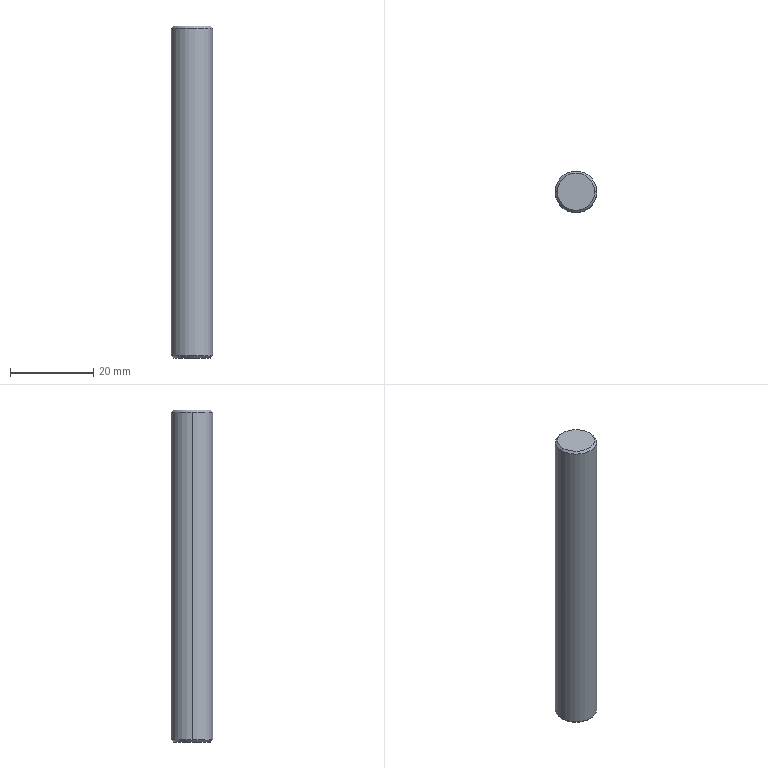Part | SolidWorks | features Chamfer 1, Extrusion 1 | 1 solid | 8 faces | box 10 x 10 x 80 mm | volume 6276 mm3 | cone 4 | cylinder 2 | plane 2 | commonest cylinder face diameters 10 x2
STEP:
#1=CARTESIAN_POINT('',(4.5,0.,80.));
#2=VERTEX_POINT('',#1);
#3=CARTESIAN_POINT('',(-4.5,0.,80.));
#4=VERTEX_POINT('',#3);
#5=CARTESIAN_POINT('',(0.,0.,80.));
#6=DIRECTION('',(0.,0.,1.));
#7=DIRECTION('',(1.,0.,0.));
#8=AXIS2_PLACEMENT_3D('',#5,#6,#7);
#9=CIRCLE('',#8,4.5);
#10=EDGE_CURVE('',#2,#4,#9,.T.);
#11=ORIENTED_EDGE('',*,*,#10,.F.);
#12=CARTESIAN_POINT('',(5.,0.,79.5));
#13=VERTEX_POINT('',#12);
#14=CARTESIAN_POINT('',(4.5,0.,80.));
#15=DIRECTION('',(0.7071,0.,-0.7071));
#16=VECTOR('',#15,1000.);
#17=LINE('',#14,#16);
#18=EDGE_CURVE('',#2,#13,#17,.T.);
#19=ORIENTED_EDGE('',*,*,#18,.T.);
#20=CARTESIAN_POINT('',(-5.,0.,79.5));
#21=VERTEX_POINT('',#20);
#22=CARTESIAN_POINT('',(0.,0.,79.5));
#23=DIRECTION('',(0.,0.,-1.));
#24=DIRECTION('',(1.,0.,0.));
#25=AXIS2_PLACEMENT_3D('',#22,#23,#24);
#26=CIRCLE('',#25,5.);
#27=EDGE_CURVE('',#21,#13,#26,.T.);
#28=ORIENTED_EDGE('',*,*,#27,.F.);
#29=CARTESIAN_POINT('',(-4.5,0.,80.));
#30=DIRECTION('',(-0.7071,0.,-0.7071));
#31=VECTOR('',#30,1000.);
#32=LINE('',#29,#31);
#33=EDGE_CURVE('',#4,#21,#32,.T.);
#34=ORIENTED_EDGE('',*,*,#33,.F.);
#35=EDGE_LOOP('',(#11,#19,#28,#34));
#36=FACE_OUTER_BOUND('',#35,.T.);
#37=CARTESIAN_POINT('',(0.,0.,80.));
#38=DIRECTION('',(0.,0.,-1.));
#39=DIRECTION('',(-1.,0.,0.));
#40=AXIS2_PLACEMENT_3D('',#37,#38,#39);
#41=CONICAL_SURFACE('',#40,4.5,0.7854);
#42=ADVANCED_FACE('',(#36),#41,.T.);
#43=CARTESIAN_POINT('',(-4.5,0.,0.));
#44=VERTEX_POINT('',#43);
#45=CARTESIAN_POINT('',(4.5,0.,0.));
#46=VERTEX_POINT('',#45);
#47=CARTESIAN_POINT('',(0.,0.,0.));
#48=DIRECTION('',(0.,0.,-1.));
#49=DIRECTION('',(1.,0.,0.));
#50=AXIS2_PLACEMENT_3D('',#47,#48,#49);
#51=CIRCLE('',#50,4.5);
#52=EDGE_CURVE('',#44,#46,#51,.T.);
#53=ORIENTED_EDGE('',*,*,#52,.F.);
#54=CARTESIAN_POINT('',(-5.,0.,0.5));
#55=VERTEX_POINT('',#54);
#56=CARTESIAN_POINT('',(-5.,0.,0.5));
#57=DIRECTION('',(-0.7071,0.,0.7071));
#58=VECTOR('',#57,1000.);
#59=LINE('',#56,#58);
#60=EDGE_CURVE('',#44,#55,#59,.T.);
#61=ORIENTED_EDGE('',*,*,#60,.T.);
#62=CARTESIAN_POINT('',(5.,0.,0.5));
#63=VERTEX_POINT('',#62);
#64=CARTESIAN_POINT('',(0.,0.,0.5));
#65=DIRECTION('',(0.,0.,1.));
#66=DIRECTION('',(1.,0.,0.));
#67=AXIS2_PLACEMENT_3D('',#64,#65,#66);
#68=CIRCLE('',#67,5.);
#69=EDGE_CURVE('',#63,#55,#68,.T.);
#70=ORIENTED_EDGE('',*,*,#69,.F.);
#71=CARTESIAN_POINT('',(5.,0.,0.5));
#72=DIRECTION('',(0.7071,0.,0.7071));
#73=VECTOR('',#72,1000.);
#74=LINE('',#71,#73);
#75=EDGE_CURVE('',#46,#63,#74,.T.);
#76=ORIENTED_EDGE('',*,*,#75,.F.);
#77=EDGE_LOOP('',(#53,#61,#70,#76));
#78=FACE_OUTER_BOUND('',#77,.T.);
#79=CARTESIAN_POINT('',(0.,0.,0.5));
#80=DIRECTION('',(0.,0.,1.));
#81=DIRECTION('',(1.,0.,0.));
#82=AXIS2_PLACEMENT_3D('',#79,#80,#81);
#83=CONICAL_SURFACE('',#82,5.,0.7854);
#84=ADVANCED_FACE('',(#78),#83,.T.);
#85=ORIENTED_EDGE('',*,*,#27,.T.);
#86=CARTESIAN_POINT('',(5.,0.,80.));
#87=DIRECTION('',(0.,0.,-1.));
#88=VECTOR('',#87,1000.);
#89=LINE('',#86,#88);
#90=EDGE_CURVE('',#13,#63,#89,.T.);
#91=ORIENTED_EDGE('',*,*,#90,.T.);
#92=ORIENTED_EDGE('',*,*,#69,.T.);
#93=CARTESIAN_POINT('',(-5.,0.,80.));
#94=DIRECTION('',(0.,0.,-1.));
#95=VECTOR('',#94,1000.);
#96=LINE('',#93,#95);
#97=EDGE_CURVE('',#21,#55,#96,.T.);
#98=ORIENTED_EDGE('',*,*,#97,.F.);
#99=EDGE_LOOP('',(#85,#91,#92,#98));
#100=FACE_OUTER_BOUND('',#99,.T.);
#101=CARTESIAN_POINT('',(0.,0.,80.));
#102=DIRECTION('',(0.,0.,-1.));
#103=DIRECTION('',(-1.,0.,0.));
#104=AXIS2_PLACEMENT_3D('',#101,#102,#103);
#105=CYLINDRICAL_SURFACE('',#104,5.);
#106=ADVANCED_FACE('',(#100),#105,.T.);
#107=ORIENTED_EDGE('',*,*,#90,.F.);
#108=CARTESIAN_POINT('',(0.,0.,79.5));
#109=DIRECTION('',(0.,0.,-1.));
#110=DIRECTION('',(1.,0.,0.));
#111=AXIS2_PLACEMENT_3D('',#108,#109,#110);
#112=CIRCLE('',#111,5.);
#113=EDGE_CURVE('',#13,#21,#112,.T.);
#114=ORIENTED_EDGE('',*,*,#113,.T.);
#115=ORIENTED_EDGE('',*,*,#97,.T.);
#116=CARTESIAN_POINT('',(0.,0.,0.5));
#117=DIRECTION('',(0.,0.,1.));
#118=DIRECTION('',(1.,0.,0.));
#119=AXIS2_PLACEMENT_3D('',#116,#117,#118);
#120=CIRCLE('',#119,5.);
#121=EDGE_CURVE('',#55,#63,#120,.T.);
#122=ORIENTED_EDGE('',*,*,#121,.T.);
#123=EDGE_LOOP('',(#107,#114,#115,#122));
#124=FACE_OUTER_BOUND('',#123,.T.);
#125=CARTESIAN_POINT('',(0.,0.,80.));
#126=DIRECTION('',(0.,0.,-1.));
#127=DIRECTION('',(-1.,0.,0.));
#128=AXIS2_PLACEMENT_3D('',#125,#126,#127);
#129=CYLINDRICAL_SURFACE('',#128,5.);
#130=ADVANCED_FACE('',(#124),#129,.T.);
#131=CARTESIAN_POINT('',(0.,0.,80.));
#132=DIRECTION('',(0.,0.,1.));
#133=DIRECTION('',(1.,0.,0.));
#134=AXIS2_PLACEMENT_3D('',#131,#132,#133);
#135=CIRCLE('',#134,4.5);
#136=EDGE_CURVE('',#4,#2,#135,.T.);
#137=ORIENTED_EDGE('',*,*,#136,.T.);
#138=ORIENTED_EDGE('',*,*,#10,.T.);
#139=EDGE_LOOP('',(#137,#138));
#140=FACE_OUTER_BOUND('',#139,.T.);
#141=CARTESIAN_POINT('',(0.,0.,80.));
#142=DIRECTION('',(0.,0.,1.));
#143=DIRECTION('',(1.,0.,0.));
#144=AXIS2_PLACEMENT_3D('',#141,#142,#143);
#145=PLANE('',#144);
#146=ADVANCED_FACE('',(#140),#145,.T.);
#147=CARTESIAN_POINT('',(0.,0.,0.));
#148=DIRECTION('',(0.,0.,-1.));
#149=DIRECTION('',(1.,0.,0.));
#150=AXIS2_PLACEMENT_3D('',#147,#148,#149);
#151=CIRCLE('',#150,4.5);
#152=EDGE_CURVE('',#46,#44,#151,.T.);
#153=ORIENTED_EDGE('',*,*,#152,.T.);
#154=ORIENTED_EDGE('',*,*,#52,.T.);
#155=EDGE_LOOP('',(#153,#154));
#156=FACE_OUTER_BOUND('',#155,.T.);
#157=CARTESIAN_POINT('',(0.,0.,0.));
#158=DIRECTION('',(0.,0.,1.));
#159=DIRECTION('',(1.,0.,0.));
#160=AXIS2_PLACEMENT_3D('',#157,#158,#159);
#161=PLANE('',#160);
#162=ADVANCED_FACE('',(#156),#161,.F.);
#163=ORIENTED_EDGE('',*,*,#60,.F.);
#164=ORIENTED_EDGE('',*,*,#152,.F.);
#165=ORIENTED_EDGE('',*,*,#75,.T.);
#166=ORIENTED_EDGE('',*,*,#121,.F.);
#167=EDGE_LOOP('',(#163,#164,#165,#166));
#168=FACE_OUTER_BOUND('',#167,.T.);
#169=CARTESIAN_POINT('',(0.,0.,0.5));
#170=DIRECTION('',(0.,0.,1.));
#171=DIRECTION('',(1.,0.,0.));
#172=AXIS2_PLACEMENT_3D('',#169,#170,#171);
#173=CONICAL_SURFACE('',#172,5.,0.7854);
#174=ADVANCED_FACE('',(#168),#173,.T.);
#175=ORIENTED_EDGE('',*,*,#18,.F.);
#176=ORIENTED_EDGE('',*,*,#136,.F.);
#177=ORIENTED_EDGE('',*,*,#33,.T.);
#178=ORIENTED_EDGE('',*,*,#113,.F.);
#179=EDGE_LOOP('',(#175,#176,#177,#178));
#180=FACE_OUTER_BOUND('',#179,.T.);
#181=CARTESIAN_POINT('',(0.,0.,80.));
#182=DIRECTION('',(0.,0.,-1.));
#183=DIRECTION('',(-1.,0.,0.));
#184=AXIS2_PLACEMENT_3D('',#181,#182,#183);
#185=CONICAL_SURFACE('',#184,4.5,0.7854);
#186=ADVANCED_FACE('',(#180),#185,.T.);
#187=CLOSED_SHELL('',(#42,#84,#106,#130,#146,#162,#174,#186));
#188=MANIFOLD_SOLID_BREP('',#187);
#189=CARTESIAN_POINT('',(0.,0.,0.));
#190=DIRECTION('',(0.,0.,1.));
#191=DIRECTION('',(1.,0.,0.));
#192=AXIS2_PLACEMENT_3D('',#189,#190,#191);
#193=(LENGTH_UNIT()NAMED_UNIT(*)SI_UNIT(.MILLI.,.METRE.));
#194=UNCERTAINTY_MEASURE_WITH_UNIT(LENGTH_MEASURE(0.00001),#193,'','');
#195=(NAMED_UNIT(*)PLANE_ANGLE_UNIT()SI_UNIT($,.RADIAN.));
#196=(NAMED_UNIT(*)SI_UNIT($,.STERADIAN.)SOLID_ANGLE_UNIT());
#197=(GEOMETRIC_REPRESENTATION_CONTEXT(3)GLOBAL_UNCERTAINTY_ASSIGNED_CONTEXT((#194))GLOBAL_UNIT_ASSIGNED_CONTEXT((#193,#195,#196))REPRESENTATION_CONTEXT('',''));
#198=ADVANCED_BREP_SHAPE_REPRESENTATION('',(#188,#192),#197);